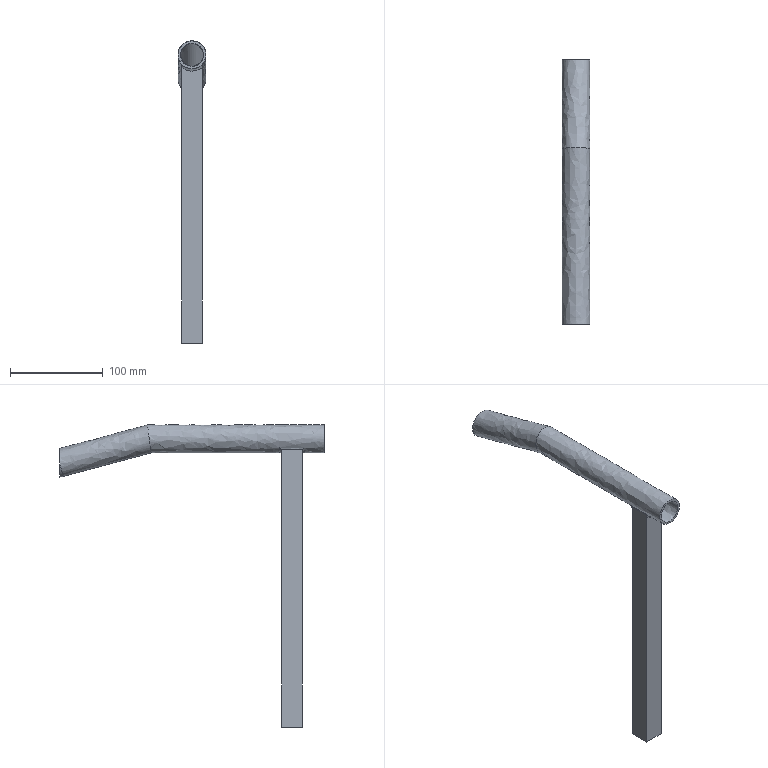Part | NX | features solid 2 | 1 solid | 22 faces | box 30 x 285.001 x 325 mm | volume 120402 mm3 | plane 11 | spline 10 | cylinder 1 | commonest cylinder face diameters 30 x1